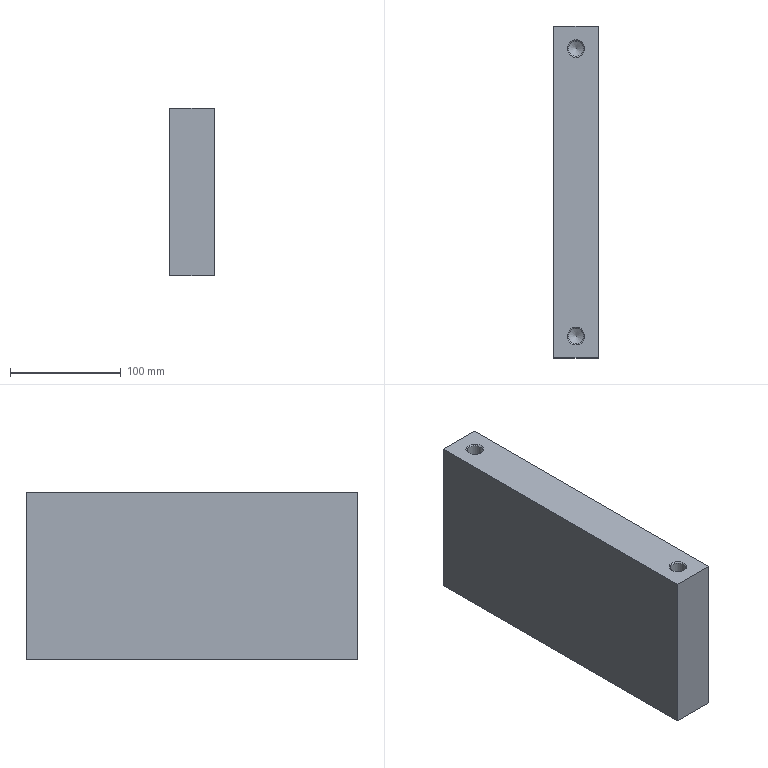Part | NX | features solid 2 | 1 solid | 15 faces | box 40 x 300 x 151.131 mm | volume 1792070 mm3 | plane 6 | cone 6 | cylinder 3 | commonest cylinder face diameters 14 x3
STEP:
#1=CARTESIAN_POINT('',(1569.977,357.095,246.13));
#2=VERTEX_POINT('',#1);
#3=CARTESIAN_POINT('',(1529.977,357.095,246.13));
#4=VERTEX_POINT('',#3);
#5=CARTESIAN_POINT('',(1344.977,357.095,246.13));
#6=DIRECTION('',(-1.,0.,0.));
#7=VECTOR('',#6,1000.);
#8=LINE('',#5,#7);
#9=EDGE_CURVE('',#2,#4,#8,.T.);
#10=ORIENTED_EDGE('',*,*,#9,.F.);
#11=CARTESIAN_POINT('',(1569.977,357.095,94.999));
#12=VERTEX_POINT('',#11);
#13=CARTESIAN_POINT('',(1569.977,357.095,159.999));
#14=DIRECTION('',(0.,0.,1.));
#15=VECTOR('',#14,1000.);
#16=LINE('',#13,#15);
#17=EDGE_CURVE('',#12,#2,#16,.T.);
#18=ORIENTED_EDGE('',*,*,#17,.F.);
#19=CARTESIAN_POINT('',(1529.977,357.095,94.999));
#20=VERTEX_POINT('',#19);
#21=CARTESIAN_POINT('',(1344.977,357.095,94.999));
#22=DIRECTION('',(-1.,0.,0.));
#23=VECTOR('',#22,1000.);
#24=LINE('',#21,#23);
#25=EDGE_CURVE('',#20,#12,#24,.F.);
#26=ORIENTED_EDGE('',*,*,#25,.F.);
#27=CARTESIAN_POINT('',(1529.977,357.095,159.999));
#28=DIRECTION('',(0.,0.,-1.));
#29=VECTOR('',#28,1000.);
#30=LINE('',#27,#29);
#31=EDGE_CURVE('',#4,#20,#30,.T.);
#32=ORIENTED_EDGE('',*,*,#31,.F.);
#33=EDGE_LOOP('',(#10,#18,#26,#32));
#34=FACE_BOUND('',#33,.T.);
#35=CARTESIAN_POINT('',(1344.977,357.095,289.999));
#36=DIRECTION('',(0.,1.,0.));
#37=DIRECTION('',(0.,0.,1.));
#38=AXIS2_PLACEMENT_3D('',#35,#36,#37);
#39=PLANE('',#38);
#40=ADVANCED_FACE('',(#34),#39,.T.);
#41=CARTESIAN_POINT('',(1541.977,336.595,94.999));
#42=VERTEX_POINT('',#41);
#43=CARTESIAN_POINT('',(1549.977,336.595,94.999));
#44=DIRECTION('',(0.,0.,-1.));
#45=DIRECTION('',(-1.,0.,0.));
#46=AXIS2_PLACEMENT_3D('',#43,#44,#45);
#47=CIRCLE('',#46,8.);
#48=EDGE_CURVE('',#42,#42,#47,.F.);
#49=ORIENTED_EDGE('',*,*,#48,.T.);
#50=EDGE_LOOP('',(#49));
#51=FACE_BOUND('',#50,.T.);
#52=CARTESIAN_POINT('',(1569.977,57.095,94.999));
#53=VERTEX_POINT('',#52);
#54=CARTESIAN_POINT('',(1569.977,6.94,94.999));
#55=DIRECTION('',(0.,1.,0.));
#56=VECTOR('',#55,1000.);
#57=LINE('',#54,#56);
#58=EDGE_CURVE('',#12,#53,#57,.F.);
#59=ORIENTED_EDGE('',*,*,#58,.T.);
#60=CARTESIAN_POINT('',(1529.977,57.095,94.999));
#61=VERTEX_POINT('',#60);
#62=CARTESIAN_POINT('',(1478.881,57.095,94.999));
#63=DIRECTION('',(-1.,0.,0.));
#64=VECTOR('',#63,1000.);
#65=LINE('',#62,#64);
#66=EDGE_CURVE('',#61,#53,#65,.F.);
#67=ORIENTED_EDGE('',*,*,#66,.F.);
#68=CARTESIAN_POINT('',(1529.977,6.94,94.999));
#69=DIRECTION('',(0.,-1.,0.));
#70=VECTOR('',#69,1000.);
#71=LINE('',#68,#70);
#72=EDGE_CURVE('',#61,#20,#71,.F.);
#73=ORIENTED_EDGE('',*,*,#72,.T.);
#74=ORIENTED_EDGE('',*,*,#25,.T.);
#75=EDGE_LOOP('',(#59,#67,#73,#74));
#76=FACE_BOUND('',#75,.T.);
#77=CARTESIAN_POINT('',(1364.955,6.94,94.999));
#78=DIRECTION('',(0.,0.,-1.));
#79=DIRECTION('',(-1.,0.,0.));
#80=AXIS2_PLACEMENT_3D('',#77,#78,#79);
#81=PLANE('',#80);
#82=ADVANCED_FACE('',(#51,#76),#81,.T.);
#83=CARTESIAN_POINT('',(1541.977,76.595,246.13));
#84=VERTEX_POINT('',#83);
#85=CARTESIAN_POINT('',(1549.977,76.595,246.13));
#86=DIRECTION('',(0.,0.,-1.));
#87=DIRECTION('',(-1.,0.,0.));
#88=AXIS2_PLACEMENT_3D('',#85,#86,#87);
#89=CIRCLE('',#88,8.);
#90=EDGE_CURVE('',#84,#84,#89,.T.);
#91=ORIENTED_EDGE('',*,*,#90,.T.);
#92=EDGE_LOOP('',(#91));
#93=FACE_BOUND('',#92,.T.);
#94=CARTESIAN_POINT('',(1541.977,336.595,246.13));
#95=VERTEX_POINT('',#94);
#96=CARTESIAN_POINT('',(1549.977,336.595,246.13));
#97=DIRECTION('',(0.,0.,-1.));
#98=DIRECTION('',(-1.,0.,0.));
#99=AXIS2_PLACEMENT_3D('',#96,#97,#98);
#100=CIRCLE('',#99,8.);
#101=EDGE_CURVE('',#95,#95,#100,.T.);
#102=ORIENTED_EDGE('',*,*,#101,.T.);
#103=EDGE_LOOP('',(#102));
#104=FACE_BOUND('',#103,.T.);
#105=CARTESIAN_POINT('',(1529.977,57.095,246.13));
#106=VERTEX_POINT('',#105);
#107=CARTESIAN_POINT('',(1529.977,4.191,246.13));
#108=DIRECTION('',(0.,1.,0.));
#109=VECTOR('',#108,1000.);
#110=LINE('',#107,#109);
#111=EDGE_CURVE('',#106,#4,#110,.T.);
#112=ORIENTED_EDGE('',*,*,#111,.F.);
#113=CARTESIAN_POINT('',(1569.977,57.095,246.13));
#114=VERTEX_POINT('',#113);
#115=CARTESIAN_POINT('',(3499.955,57.095,246.13));
#116=DIRECTION('',(1.,0.,0.));
#117=VECTOR('',#116,1000.);
#118=LINE('',#115,#117);
#119=EDGE_CURVE('',#106,#114,#118,.T.);
#120=ORIENTED_EDGE('',*,*,#119,.T.);
#121=CARTESIAN_POINT('',(1569.977,4.191,246.13));
#122=DIRECTION('',(0.,-1.,0.));
#123=VECTOR('',#122,1000.);
#124=LINE('',#121,#123);
#125=EDGE_CURVE('',#2,#114,#124,.T.);
#126=ORIENTED_EDGE('',*,*,#125,.F.);
#127=ORIENTED_EDGE('',*,*,#9,.T.);
#128=EDGE_LOOP('',(#112,#120,#126,#127));
#129=FACE_BOUND('',#128,.T.);
#130=CARTESIAN_POINT('',(3499.955,4.191,246.13));
#131=DIRECTION('',(0.,0.,-1.));
#132=DIRECTION('',(1.,0.,0.));
#133=AXIS2_PLACEMENT_3D('',#130,#131,#132);
#134=PLANE('',#133);
#135=ADVANCED_FACE('',(#93,#104,#129),#134,.F.);
#136=CARTESIAN_POINT('',(1529.977,57.095,159.999));
#137=DIRECTION('',(0.,0.,-1.));
#138=VECTOR('',#137,1000.);
#139=LINE('',#136,#138);
#140=EDGE_CURVE('',#106,#61,#139,.T.);
#141=ORIENTED_EDGE('',*,*,#140,.F.);
#142=ORIENTED_EDGE('',*,*,#111,.T.);
#143=ORIENTED_EDGE('',*,*,#31,.T.);
#144=ORIENTED_EDGE('',*,*,#72,.F.);
#145=EDGE_LOOP('',(#141,#142,#143,#144));
#146=FACE_BOUND('',#145,.T.);
#147=CARTESIAN_POINT('',(1529.977,2.095,159.999));
#148=DIRECTION('',(-1.,0.,0.));
#149=DIRECTION('',(0.,0.,1.));
#150=AXIS2_PLACEMENT_3D('',#147,#148,#149);
#151=PLANE('',#150);
#152=ADVANCED_FACE('',(#146),#151,.T.);
#153=CARTESIAN_POINT('',(1569.977,57.095,149.065));
#154=DIRECTION('',(0.,0.,-1.));
#155=VECTOR('',#154,1000.);
#156=LINE('',#153,#155);
#157=EDGE_CURVE('',#114,#53,#156,.T.);
#158=ORIENTED_EDGE('',*,*,#157,.T.);
#159=ORIENTED_EDGE('',*,*,#58,.F.);
#160=ORIENTED_EDGE('',*,*,#17,.T.);
#161=ORIENTED_EDGE('',*,*,#125,.T.);
#162=EDGE_LOOP('',(#158,#159,#160,#161));
#163=FACE_BOUND('',#162,.T.);
#164=CARTESIAN_POINT('',(1569.977,2.095,159.999));
#165=DIRECTION('',(1.,0.,0.));
#166=DIRECTION('',(0.,0.,-1.));
#167=AXIS2_PLACEMENT_3D('',#164,#165,#166);
#168=PLANE('',#167);
#169=ADVANCED_FACE('',(#163),#168,.T.);
#170=ORIENTED_EDGE('',*,*,#157,.F.);
#171=ORIENTED_EDGE('',*,*,#119,.F.);
#172=ORIENTED_EDGE('',*,*,#140,.T.);
#173=ORIENTED_EDGE('',*,*,#66,.T.);
#174=EDGE_LOOP('',(#170,#171,#172,#173));
#175=FACE_BOUND('',#174,.T.);
#176=CARTESIAN_POINT('',(1478.881,57.095,149.065));
#177=DIRECTION('',(0.,1.,0.));
#178=DIRECTION('',(0.,0.,-1.));
#179=AXIS2_PLACEMENT_3D('',#176,#177,#178);
#180=PLANE('',#179);
#181=ADVANCED_FACE('',(#175),#180,.F.);
#182=CARTESIAN_POINT('',(1556.977,336.595,139.999));
#183=VERTEX_POINT('',#182);
#184=CARTESIAN_POINT('',(1549.977,336.595,139.999));
#185=DIRECTION('',(0.,0.,1.));
#186=DIRECTION('',(1.,0.,0.));
#187=AXIS2_PLACEMENT_3D('',#184,#185,#186);
#188=CIRCLE('',#187,7.);
#189=EDGE_CURVE('',#183,#183,#188,.F.);
#190=ORIENTED_EDGE('',*,*,#189,.T.);
#191=EDGE_LOOP('',(#190));
#192=FACE_BOUND('',#191,.T.);
#193=CARTESIAN_POINT('',(1549.977,336.595,144.205));
#194=VERTEX_POINT('',#193);
#195=VERTEX_LOOP('',#194);
#196=FACE_BOUND('',#195,.T.);
#197=CARTESIAN_POINT('',(1549.977,336.595,139.999));
#198=DIRECTION('',(0.,0.,-1.));
#199=DIRECTION('',(-1.,0.,0.));
#200=AXIS2_PLACEMENT_3D('',#197,#198,#199);
#201=CONICAL_SURFACE('',#200,7.,1.03);
#202=ADVANCED_FACE('',(#192,#196),#201,.F.);
#203=CARTESIAN_POINT('',(1556.977,336.595,95.999));
#204=VERTEX_POINT('',#203);
#205=CARTESIAN_POINT('',(1549.977,336.595,95.999));
#206=DIRECTION('',(0.,0.,1.));
#207=DIRECTION('',(1.,0.,0.));
#208=AXIS2_PLACEMENT_3D('',#205,#206,#207);
#209=CIRCLE('',#208,7.);
#210=EDGE_CURVE('',#204,#204,#209,.F.);
#211=ORIENTED_EDGE('',*,*,#210,.T.);
#212=EDGE_LOOP('',(#211));
#213=FACE_BOUND('',#212,.T.);
#214=ORIENTED_EDGE('',*,*,#189,.F.);
#215=EDGE_LOOP('',(#214));
#216=FACE_BOUND('',#215,.T.);
#217=CARTESIAN_POINT('',(1549.977,336.595,94.999));
#218=DIRECTION('',(0.,0.,1.));
#219=DIRECTION('',(1.,0.,0.));
#220=AXIS2_PLACEMENT_3D('',#217,#218,#219);
#221=CYLINDRICAL_SURFACE('',#220,7.);
#222=ADVANCED_FACE('',(#213,#216),#221,.F.);
#223=ORIENTED_EDGE('',*,*,#210,.F.);
#224=EDGE_LOOP('',(#223));
#225=FACE_BOUND('',#224,.T.);
#226=ORIENTED_EDGE('',*,*,#48,.F.);
#227=EDGE_LOOP('',(#226));
#228=FACE_BOUND('',#227,.T.);
#229=CARTESIAN_POINT('',(1549.977,336.595,94.999));
#230=DIRECTION('',(0.,0.,-1.));
#231=DIRECTION('',(-1.,0.,0.));
#232=AXIS2_PLACEMENT_3D('',#229,#230,#231);
#233=CONICAL_SURFACE('',#232,8.,0.7854);
#234=ADVANCED_FACE('',(#225,#228),#233,.F.);
#235=CARTESIAN_POINT('',(1542.977,336.595,201.13));
#236=VERTEX_POINT('',#235);
#237=CARTESIAN_POINT('',(1549.977,336.595,201.13));
#238=DIRECTION('',(0.,0.,-1.));
#239=DIRECTION('',(-1.,0.,0.));
#240=AXIS2_PLACEMENT_3D('',#237,#238,#239);
#241=CIRCLE('',#240,7.);
#242=EDGE_CURVE('',#236,#236,#241,.F.);
#243=ORIENTED_EDGE('',*,*,#242,.T.);
#244=EDGE_LOOP('',(#243));
#245=FACE_BOUND('',#244,.T.);
#246=CARTESIAN_POINT('',(1549.977,336.595,196.924));
#247=VERTEX_POINT('',#246);
#248=VERTEX_LOOP('',#247);
#249=FACE_BOUND('',#248,.T.);
#250=CARTESIAN_POINT('',(1549.977,336.595,201.13));
#251=DIRECTION('',(0.,0.,1.));
#252=DIRECTION('',(1.,0.,0.));
#253=AXIS2_PLACEMENT_3D('',#250,#251,#252);
#254=CONICAL_SURFACE('',#253,7.,1.03);
#255=ADVANCED_FACE('',(#245,#249),#254,.F.);
#256=CARTESIAN_POINT('',(1542.977,336.595,245.13));
#257=VERTEX_POINT('',#256);
#258=CARTESIAN_POINT('',(1549.977,336.595,245.13));
#259=DIRECTION('',(0.,0.,-1.));
#260=DIRECTION('',(-1.,0.,0.));
#261=AXIS2_PLACEMENT_3D('',#258,#259,#260);
#262=CIRCLE('',#261,7.);
#263=EDGE_CURVE('',#257,#257,#262,.F.);
#264=ORIENTED_EDGE('',*,*,#263,.T.);
#265=EDGE_LOOP('',(#264));
#266=FACE_BOUND('',#265,.T.);
#267=ORIENTED_EDGE('',*,*,#242,.F.);
#268=EDGE_LOOP('',(#267));
#269=FACE_BOUND('',#268,.T.);
#270=CARTESIAN_POINT('',(1549.977,336.595,246.13));
#271=DIRECTION('',(0.,0.,-1.));
#272=DIRECTION('',(-1.,0.,0.));
#273=AXIS2_PLACEMENT_3D('',#270,#271,#272);
#274=CYLINDRICAL_SURFACE('',#273,7.);
#275=ADVANCED_FACE('',(#266,#269),#274,.F.);
#276=ORIENTED_EDGE('',*,*,#263,.F.);
#277=EDGE_LOOP('',(#276));
#278=FACE_BOUND('',#277,.T.);
#279=ORIENTED_EDGE('',*,*,#101,.F.);
#280=EDGE_LOOP('',(#279));
#281=FACE_BOUND('',#280,.T.);
#282=CARTESIAN_POINT('',(1549.977,336.595,246.13));
#283=DIRECTION('',(0.,0.,1.));
#284=DIRECTION('',(1.,0.,0.));
#285=AXIS2_PLACEMENT_3D('',#282,#283,#284);
#286=CONICAL_SURFACE('',#285,8.,0.7854);
#287=ADVANCED_FACE('',(#278,#281),#286,.F.);
#288=CARTESIAN_POINT('',(1542.977,76.595,201.13));
#289=VERTEX_POINT('',#288);
#290=CARTESIAN_POINT('',(1549.977,76.595,201.13));
#291=DIRECTION('',(0.,0.,-1.));
#292=DIRECTION('',(-1.,0.,0.));
#293=AXIS2_PLACEMENT_3D('',#290,#291,#292);
#294=CIRCLE('',#293,7.);
#295=EDGE_CURVE('',#289,#289,#294,.F.);
#296=ORIENTED_EDGE('',*,*,#295,.T.);
#297=EDGE_LOOP('',(#296));
#298=FACE_BOUND('',#297,.T.);
#299=CARTESIAN_POINT('',(1549.977,76.595,196.924));
#300=VERTEX_POINT('',#299);
#301=VERTEX_LOOP('',#300);
#302=FACE_BOUND('',#301,.T.);
#303=CARTESIAN_POINT('',(1549.977,76.595,201.13));
#304=DIRECTION('',(0.,0.,1.));
#305=DIRECTION('',(1.,0.,0.));
#306=AXIS2_PLACEMENT_3D('',#303,#304,#305);
#307=CONICAL_SURFACE('',#306,7.,1.03);
#308=ADVANCED_FACE('',(#298,#302),#307,.F.);
#309=CARTESIAN_POINT('',(1542.977,76.595,245.13));
#310=VERTEX_POINT('',#309);
#311=CARTESIAN_POINT('',(1549.977,76.595,245.13));
#312=DIRECTION('',(0.,0.,-1.));
#313=DIRECTION('',(-1.,0.,0.));
#314=AXIS2_PLACEMENT_3D('',#311,#312,#313);
#315=CIRCLE('',#314,7.);
#316=EDGE_CURVE('',#310,#310,#315,.F.);
#317=ORIENTED_EDGE('',*,*,#316,.T.);
#318=EDGE_LOOP('',(#317));
#319=FACE_BOUND('',#318,.T.);
#320=ORIENTED_EDGE('',*,*,#295,.F.);
#321=EDGE_LOOP('',(#320));
#322=FACE_BOUND('',#321,.T.);
#323=CARTESIAN_POINT('',(1549.977,76.595,246.13));
#324=DIRECTION('',(0.,0.,-1.));
#325=DIRECTION('',(-1.,0.,0.));
#326=AXIS2_PLACEMENT_3D('',#323,#324,#325);
#327=CYLINDRICAL_SURFACE('',#326,7.);
#328=ADVANCED_FACE('',(#319,#322),#327,.F.);
#329=ORIENTED_EDGE('',*,*,#316,.F.);
#330=EDGE_LOOP('',(#329));
#331=FACE_BOUND('',#330,.T.);
#332=ORIENTED_EDGE('',*,*,#90,.F.);
#333=EDGE_LOOP('',(#332));
#334=FACE_BOUND('',#333,.T.);
#335=CARTESIAN_POINT('',(1549.977,76.595,246.13));
#336=DIRECTION('',(0.,0.,1.));
#337=DIRECTION('',(1.,0.,0.));
#338=AXIS2_PLACEMENT_3D('',#335,#336,#337);
#339=CONICAL_SURFACE('',#338,8.,0.7854);
#340=ADVANCED_FACE('',(#331,#334),#339,.F.);
#341=CLOSED_SHELL('',(#40,#82,#135,#152,#169,#181,#202,#222,#234,#255,#275,#287,#308,#328,#340));
#342=MANIFOLD_SOLID_BREP('',#341);
#343=(LENGTH_UNIT()NAMED_UNIT(*)SI_UNIT(.MILLI.,.METRE.));
#344=UNCERTAINTY_MEASURE_WITH_UNIT(LENGTH_MEASURE(0.00001),#343,'','');
#345=(NAMED_UNIT(*)PLANE_ANGLE_UNIT()SI_UNIT($,.RADIAN.));
#346=(NAMED_UNIT(*)SI_UNIT($,.STERADIAN.)SOLID_ANGLE_UNIT());
#347=(GEOMETRIC_REPRESENTATION_CONTEXT(3)GLOBAL_UNCERTAINTY_ASSIGNED_CONTEXT((#344))GLOBAL_UNIT_ASSIGNED_CONTEXT((#343,#345,#346))REPRESENTATION_CONTEXT('',''));
#348=ADVANCED_BREP_SHAPE_REPRESENTATION('',(#342),#347);